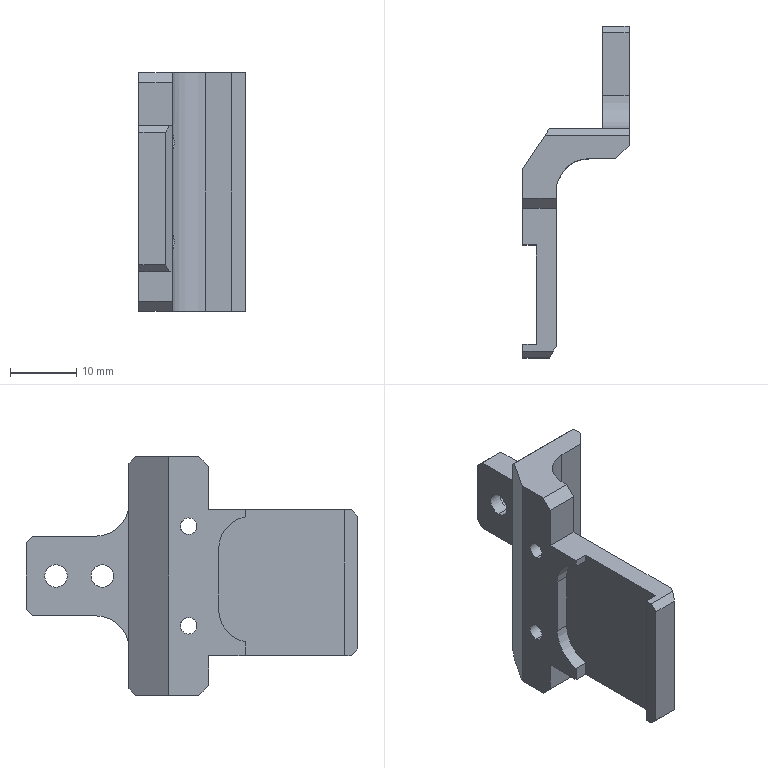Part | STEP file | 0-19 Finger 1 | 1 solid | 52 faces | box 16 x 50 x 36 mm | volume 5853 mm3 | plane 35 | cylinder 17 | commonest cylinder face diameters 10 x5 2.5 x4 3.4 x4 6 x4